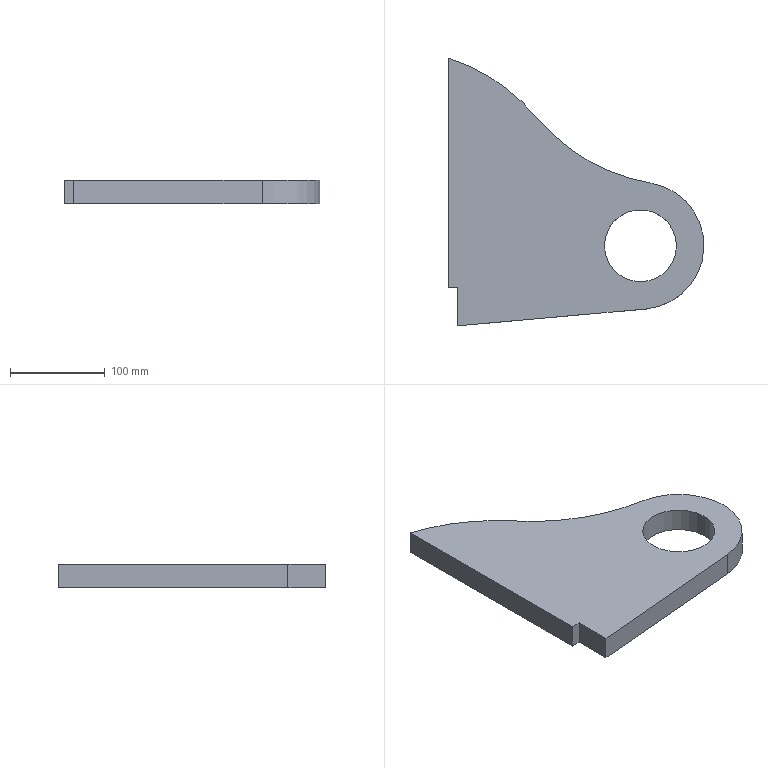Part | SolidWorks | features Extrusion 1 | 1 solid | 11 faces | box 270 x 282.5 x 25 mm | volume 1101150 mm3 | plane 6 | cylinder 5 | commonest cylinder face diameters 76 x2 400 x2 134 x1
STEP:
#1=CARTESIAN_POINT('',(-38.,0.,25.));
#2=VERTEX_POINT('',#1);
#3=CARTESIAN_POINT('',(38.,0.,25.));
#4=VERTEX_POINT('',#3);
#5=CARTESIAN_POINT('',(0.,0.,25.));
#6=DIRECTION('',(0.,0.,1.));
#7=DIRECTION('',(1.,0.,0.));
#8=AXIS2_PLACEMENT_3D('',#5,#6,#7);
#9=CIRCLE('',#8,38.);
#10=EDGE_CURVE('',#2,#4,#9,.T.);
#11=ORIENTED_EDGE('',*,*,#10,.T.);
#12=CARTESIAN_POINT('',(38.,0.,0.));
#13=VERTEX_POINT('',#12);
#14=CARTESIAN_POINT('',(38.,0.,25.));
#15=DIRECTION('',(0.,0.,-1.));
#16=VECTOR('',#15,1000.);
#17=LINE('',#14,#16);
#18=EDGE_CURVE('',#4,#13,#17,.T.);
#19=ORIENTED_EDGE('',*,*,#18,.T.);
#20=CARTESIAN_POINT('',(-38.,0.,0.));
#21=VERTEX_POINT('',#20);
#22=CARTESIAN_POINT('',(0.,0.,0.));
#23=DIRECTION('',(0.,0.,1.));
#24=DIRECTION('',(1.,0.,0.));
#25=AXIS2_PLACEMENT_3D('',#22,#23,#24);
#26=CIRCLE('',#25,38.);
#27=EDGE_CURVE('',#21,#13,#26,.T.);
#28=ORIENTED_EDGE('',*,*,#27,.F.);
#29=CARTESIAN_POINT('',(-38.,0.,25.));
#30=DIRECTION('',(0.,0.,-1.));
#31=VECTOR('',#30,1000.);
#32=LINE('',#29,#31);
#33=EDGE_CURVE('',#2,#21,#32,.T.);
#34=ORIENTED_EDGE('',*,*,#33,.F.);
#35=EDGE_LOOP('',(#11,#19,#28,#34));
#36=FACE_OUTER_BOUND('',#35,.T.);
#37=CARTESIAN_POINT('',(0.,0.,25.));
#38=DIRECTION('',(0.,0.,-1.));
#39=DIRECTION('',(-1.,0.,0.));
#40=AXIS2_PLACEMENT_3D('',#37,#38,#39);
#41=CYLINDRICAL_SURFACE('',#40,38.);
#42=ADVANCED_FACE('',(#36),#41,.F.);
#43=CARTESIAN_POINT('',(-109.363,135.258,25.));
#44=VERTEX_POINT('',#43);
#45=CARTESIAN_POINT('',(-203.,198.,25.));
#46=VERTEX_POINT('',#45);
#47=CARTESIAN_POINT('',(-263.,7.212,25.));
#48=DIRECTION('',(0.,0.,1.));
#49=DIRECTION('',(1.,0.,0.));
#50=AXIS2_PLACEMENT_3D('',#47,#48,#49);
#51=CIRCLE('',#50,200.);
#52=EDGE_CURVE('',#44,#46,#51,.T.);
#53=ORIENTED_EDGE('',*,*,#52,.T.);
#54=CARTESIAN_POINT('',(-203.,-44.5,25.));
#55=VERTEX_POINT('',#54);
#56=CARTESIAN_POINT('',(-203.,198.,25.));
#57=DIRECTION('',(0.,-1.,0.));
#58=VECTOR('',#57,1000.);
#59=LINE('',#56,#58);
#60=EDGE_CURVE('',#46,#55,#59,.T.);
#61=ORIENTED_EDGE('',*,*,#60,.T.);
#62=CARTESIAN_POINT('',(-193.,-44.5,25.));
#63=VERTEX_POINT('',#62);
#64=CARTESIAN_POINT('',(-203.,-44.5,25.));
#65=DIRECTION('',(1.,0.,0.));
#66=VECTOR('',#65,1000.);
#67=LINE('',#64,#66);
#68=EDGE_CURVE('',#55,#63,#67,.T.);
#69=ORIENTED_EDGE('',*,*,#68,.T.);
#70=CARTESIAN_POINT('',(-193.,-84.5,25.));
#71=VERTEX_POINT('',#70);
#72=CARTESIAN_POINT('',(-193.,-44.5,25.));
#73=DIRECTION('',(0.,-1.,0.));
#74=VECTOR('',#73,1000.);
#75=LINE('',#72,#74);
#76=EDGE_CURVE('',#63,#71,#75,.T.);
#77=ORIENTED_EDGE('',*,*,#76,.T.);
#78=CARTESIAN_POINT('',(5.959,-66.734,25.));
#79=VERTEX_POINT('',#78);
#80=CARTESIAN_POINT('',(-193.,-84.5,25.));
#81=DIRECTION('',(0.996,0.08894,0.));
#82=VECTOR('',#81,1000.);
#83=LINE('',#80,#82);
#84=EDGE_CURVE('',#71,#79,#83,.T.);
#85=ORIENTED_EDGE('',*,*,#84,.T.);
#86=CARTESIAN_POINT('',(11.11,66.072,25.));
#87=VERTEX_POINT('',#86);
#88=CARTESIAN_POINT('',(0.,0.,25.));
#89=DIRECTION('',(0.,0.,1.));
#90=DIRECTION('',(1.,0.,0.));
#91=AXIS2_PLACEMENT_3D('',#88,#89,#90);
#92=CIRCLE('',#91,67.);
#93=EDGE_CURVE('',#79,#87,#92,.T.);
#94=ORIENTED_EDGE('',*,*,#93,.T.);
#95=CARTESIAN_POINT('',(44.274,263.304,25.));
#96=DIRECTION('',(0.,0.,-1.));
#97=DIRECTION('',(1.,0.,0.));
#98=AXIS2_PLACEMENT_3D('',#95,#96,#97);
#99=CIRCLE('',#98,200.);
#100=EDGE_CURVE('',#87,#44,#99,.T.);
#101=ORIENTED_EDGE('',*,*,#100,.T.);
#102=EDGE_LOOP('',(#53,#61,#69,#77,#85,#94,#101));
#103=FACE_OUTER_BOUND('',#102,.T.);
#104=ORIENTED_EDGE('',*,*,#10,.F.);
#105=CARTESIAN_POINT('',(0.,0.,25.));
#106=DIRECTION('',(0.,0.,1.));
#107=DIRECTION('',(1.,0.,0.));
#108=AXIS2_PLACEMENT_3D('',#105,#106,#107);
#109=CIRCLE('',#108,38.);
#110=EDGE_CURVE('',#4,#2,#109,.T.);
#111=ORIENTED_EDGE('',*,*,#110,.F.);
#112=EDGE_LOOP('',(#104,#111));
#113=FACE_BOUND('',#112,.T.);
#114=CARTESIAN_POINT('',(-263.,7.212,25.));
#115=DIRECTION('',(0.,0.,1.));
#116=DIRECTION('',(1.,0.,0.));
#117=AXIS2_PLACEMENT_3D('',#114,#115,#116);
#118=PLANE('',#117);
#119=ADVANCED_FACE('',(#103,#113),#118,.T.);
#120=CARTESIAN_POINT('',(-109.363,135.258,0.));
#121=VERTEX_POINT('',#120);
#122=CARTESIAN_POINT('',(-203.,198.,0.));
#123=VERTEX_POINT('',#122);
#124=CARTESIAN_POINT('',(-263.,7.212,0.));
#125=DIRECTION('',(0.,0.,1.));
#126=DIRECTION('',(1.,0.,0.));
#127=AXIS2_PLACEMENT_3D('',#124,#125,#126);
#128=CIRCLE('',#127,200.);
#129=EDGE_CURVE('',#121,#123,#128,.T.);
#130=ORIENTED_EDGE('',*,*,#129,.F.);
#131=CARTESIAN_POINT('',(11.11,66.072,0.));
#132=VERTEX_POINT('',#131);
#133=CARTESIAN_POINT('',(44.274,263.304,0.));
#134=DIRECTION('',(0.,0.,-1.));
#135=DIRECTION('',(1.,0.,0.));
#136=AXIS2_PLACEMENT_3D('',#133,#134,#135);
#137=CIRCLE('',#136,200.);
#138=EDGE_CURVE('',#132,#121,#137,.T.);
#139=ORIENTED_EDGE('',*,*,#138,.F.);
#140=CARTESIAN_POINT('',(5.959,-66.734,0.));
#141=VERTEX_POINT('',#140);
#142=CARTESIAN_POINT('',(0.,0.,0.));
#143=DIRECTION('',(0.,0.,1.));
#144=DIRECTION('',(1.,0.,0.));
#145=AXIS2_PLACEMENT_3D('',#142,#143,#144);
#146=CIRCLE('',#145,67.);
#147=EDGE_CURVE('',#141,#132,#146,.T.);
#148=ORIENTED_EDGE('',*,*,#147,.F.);
#149=CARTESIAN_POINT('',(-193.,-84.5,0.));
#150=VERTEX_POINT('',#149);
#151=CARTESIAN_POINT('',(-193.,-84.5,0.));
#152=DIRECTION('',(0.996,0.08894,0.));
#153=VECTOR('',#152,1000.);
#154=LINE('',#151,#153);
#155=EDGE_CURVE('',#150,#141,#154,.T.);
#156=ORIENTED_EDGE('',*,*,#155,.F.);
#157=CARTESIAN_POINT('',(-193.,-44.5,0.));
#158=VERTEX_POINT('',#157);
#159=CARTESIAN_POINT('',(-193.,-44.5,0.));
#160=DIRECTION('',(0.,-1.,0.));
#161=VECTOR('',#160,1000.);
#162=LINE('',#159,#161);
#163=EDGE_CURVE('',#158,#150,#162,.T.);
#164=ORIENTED_EDGE('',*,*,#163,.F.);
#165=CARTESIAN_POINT('',(-203.,-44.5,0.));
#166=VERTEX_POINT('',#165);
#167=CARTESIAN_POINT('',(-203.,-44.5,0.));
#168=DIRECTION('',(1.,0.,0.));
#169=VECTOR('',#168,1000.);
#170=LINE('',#167,#169);
#171=EDGE_CURVE('',#166,#158,#170,.T.);
#172=ORIENTED_EDGE('',*,*,#171,.F.);
#173=CARTESIAN_POINT('',(-203.,198.,0.));
#174=DIRECTION('',(0.,-1.,0.));
#175=VECTOR('',#174,1000.);
#176=LINE('',#173,#175);
#177=EDGE_CURVE('',#123,#166,#176,.T.);
#178=ORIENTED_EDGE('',*,*,#177,.F.);
#179=EDGE_LOOP('',(#130,#139,#148,#156,#164,#172,#178));
#180=FACE_OUTER_BOUND('',#179,.T.);
#181=ORIENTED_EDGE('',*,*,#27,.T.);
#182=CARTESIAN_POINT('',(0.,0.,0.));
#183=DIRECTION('',(0.,0.,1.));
#184=DIRECTION('',(1.,0.,0.));
#185=AXIS2_PLACEMENT_3D('',#182,#183,#184);
#186=CIRCLE('',#185,38.);
#187=EDGE_CURVE('',#13,#21,#186,.T.);
#188=ORIENTED_EDGE('',*,*,#187,.T.);
#189=EDGE_LOOP('',(#181,#188));
#190=FACE_BOUND('',#189,.T.);
#191=CARTESIAN_POINT('',(-263.,7.212,0.));
#192=DIRECTION('',(0.,0.,1.));
#193=DIRECTION('',(1.,0.,0.));
#194=AXIS2_PLACEMENT_3D('',#191,#192,#193);
#195=PLANE('',#194);
#196=ADVANCED_FACE('',(#180,#190),#195,.F.);
#197=ORIENTED_EDGE('',*,*,#129,.T.);
#198=CARTESIAN_POINT('',(-203.,198.,25.));
#199=DIRECTION('',(0.,0.,-1.));
#200=VECTOR('',#199,1000.);
#201=LINE('',#198,#200);
#202=EDGE_CURVE('',#46,#123,#201,.T.);
#203=ORIENTED_EDGE('',*,*,#202,.F.);
#204=ORIENTED_EDGE('',*,*,#52,.F.);
#205=CARTESIAN_POINT('',(-109.363,135.258,25.));
#206=DIRECTION('',(0.,0.,-1.));
#207=VECTOR('',#206,1000.);
#208=LINE('',#205,#207);
#209=EDGE_CURVE('',#44,#121,#208,.T.);
#210=ORIENTED_EDGE('',*,*,#209,.T.);
#211=EDGE_LOOP('',(#197,#203,#204,#210));
#212=FACE_OUTER_BOUND('',#211,.T.);
#213=CARTESIAN_POINT('',(-263.,7.212,25.));
#214=DIRECTION('',(0.,0.,-1.));
#215=DIRECTION('',(-1.,0.,0.));
#216=AXIS2_PLACEMENT_3D('',#213,#214,#215);
#217=CYLINDRICAL_SURFACE('',#216,200.);
#218=ADVANCED_FACE('',(#212),#217,.T.);
#219=ORIENTED_EDGE('',*,*,#177,.T.);
#220=CARTESIAN_POINT('',(-203.,-44.5,25.));
#221=DIRECTION('',(0.,0.,-1.));
#222=VECTOR('',#221,1000.);
#223=LINE('',#220,#222);
#224=EDGE_CURVE('',#55,#166,#223,.T.);
#225=ORIENTED_EDGE('',*,*,#224,.F.);
#226=ORIENTED_EDGE('',*,*,#60,.F.);
#227=ORIENTED_EDGE('',*,*,#202,.T.);
#228=EDGE_LOOP('',(#219,#225,#226,#227));
#229=FACE_OUTER_BOUND('',#228,.T.);
#230=CARTESIAN_POINT('',(-203.,198.,25.));
#231=DIRECTION('',(1.,0.,0.));
#232=DIRECTION('',(0.,1.,0.));
#233=AXIS2_PLACEMENT_3D('',#230,#231,#232);
#234=PLANE('',#233);
#235=ADVANCED_FACE('',(#229),#234,.F.);
#236=ORIENTED_EDGE('',*,*,#171,.T.);
#237=CARTESIAN_POINT('',(-193.,-44.5,25.));
#238=DIRECTION('',(0.,0.,-1.));
#239=VECTOR('',#238,1000.);
#240=LINE('',#237,#239);
#241=EDGE_CURVE('',#63,#158,#240,.T.);
#242=ORIENTED_EDGE('',*,*,#241,.F.);
#243=ORIENTED_EDGE('',*,*,#68,.F.);
#244=ORIENTED_EDGE('',*,*,#224,.T.);
#245=EDGE_LOOP('',(#236,#242,#243,#244));
#246=FACE_OUTER_BOUND('',#245,.T.);
#247=CARTESIAN_POINT('',(-203.,-44.5,25.));
#248=DIRECTION('',(0.,1.,0.));
#249=DIRECTION('',(0.,0.,1.));
#250=AXIS2_PLACEMENT_3D('',#247,#248,#249);
#251=PLANE('',#250);
#252=ADVANCED_FACE('',(#246),#251,.F.);
#253=ORIENTED_EDGE('',*,*,#163,.T.);
#254=CARTESIAN_POINT('',(-193.,-84.5,25.));
#255=DIRECTION('',(0.,0.,-1.));
#256=VECTOR('',#255,1000.);
#257=LINE('',#254,#256);
#258=EDGE_CURVE('',#71,#150,#257,.T.);
#259=ORIENTED_EDGE('',*,*,#258,.F.);
#260=ORIENTED_EDGE('',*,*,#76,.F.);
#261=ORIENTED_EDGE('',*,*,#241,.T.);
#262=EDGE_LOOP('',(#253,#259,#260,#261));
#263=FACE_OUTER_BOUND('',#262,.T.);
#264=CARTESIAN_POINT('',(-193.,-44.5,25.));
#265=DIRECTION('',(1.,0.,0.));
#266=DIRECTION('',(0.,0.,-1.));
#267=AXIS2_PLACEMENT_3D('',#264,#265,#266);
#268=PLANE('',#267);
#269=ADVANCED_FACE('',(#263),#268,.F.);
#270=ORIENTED_EDGE('',*,*,#155,.T.);
#271=CARTESIAN_POINT('',(5.959,-66.734,25.));
#272=DIRECTION('',(0.,0.,-1.));
#273=VECTOR('',#272,1000.);
#274=LINE('',#271,#273);
#275=EDGE_CURVE('',#79,#141,#274,.T.);
#276=ORIENTED_EDGE('',*,*,#275,.F.);
#277=ORIENTED_EDGE('',*,*,#84,.F.);
#278=ORIENTED_EDGE('',*,*,#258,.T.);
#279=EDGE_LOOP('',(#270,#276,#277,#278));
#280=FACE_OUTER_BOUND('',#279,.T.);
#281=CARTESIAN_POINT('',(-193.,-84.5,25.));
#282=DIRECTION('',(-0.08894,0.996,0.));
#283=DIRECTION('',(-0.996,-0.08894,0.));
#284=AXIS2_PLACEMENT_3D('',#281,#282,#283);
#285=PLANE('',#284);
#286=ADVANCED_FACE('',(#280),#285,.F.);
#287=ORIENTED_EDGE('',*,*,#147,.T.);
#288=CARTESIAN_POINT('',(11.11,66.072,25.));
#289=DIRECTION('',(0.,0.,-1.));
#290=VECTOR('',#289,1000.);
#291=LINE('',#288,#290);
#292=EDGE_CURVE('',#87,#132,#291,.T.);
#293=ORIENTED_EDGE('',*,*,#292,.F.);
#294=ORIENTED_EDGE('',*,*,#93,.F.);
#295=ORIENTED_EDGE('',*,*,#275,.T.);
#296=EDGE_LOOP('',(#287,#293,#294,#295));
#297=FACE_OUTER_BOUND('',#296,.T.);
#298=CARTESIAN_POINT('',(0.,0.,25.));
#299=DIRECTION('',(0.,0.,-1.));
#300=DIRECTION('',(-1.,0.,0.));
#301=AXIS2_PLACEMENT_3D('',#298,#299,#300);
#302=CYLINDRICAL_SURFACE('',#301,67.);
#303=ADVANCED_FACE('',(#297),#302,.T.);
#304=ORIENTED_EDGE('',*,*,#138,.T.);
#305=ORIENTED_EDGE('',*,*,#209,.F.);
#306=ORIENTED_EDGE('',*,*,#100,.F.);
#307=ORIENTED_EDGE('',*,*,#292,.T.);
#308=EDGE_LOOP('',(#304,#305,#306,#307));
#309=FACE_OUTER_BOUND('',#308,.T.);
#310=CARTESIAN_POINT('',(44.274,263.304,25.));
#311=DIRECTION('',(0.,0.,-1.));
#312=DIRECTION('',(-1.,0.,0.));
#313=AXIS2_PLACEMENT_3D('',#310,#311,#312);
#314=CYLINDRICAL_SURFACE('',#313,200.);
#315=ADVANCED_FACE('',(#309),#314,.F.);
#316=ORIENTED_EDGE('',*,*,#18,.F.);
#317=ORIENTED_EDGE('',*,*,#110,.T.);
#318=ORIENTED_EDGE('',*,*,#33,.T.);
#319=ORIENTED_EDGE('',*,*,#187,.F.);
#320=EDGE_LOOP('',(#316,#317,#318,#319));
#321=FACE_OUTER_BOUND('',#320,.T.);
#322=CARTESIAN_POINT('',(0.,0.,25.));
#323=DIRECTION('',(0.,0.,-1.));
#324=DIRECTION('',(-1.,0.,0.));
#325=AXIS2_PLACEMENT_3D('',#322,#323,#324);
#326=CYLINDRICAL_SURFACE('',#325,38.);
#327=ADVANCED_FACE('',(#321),#326,.F.);
#328=CLOSED_SHELL('',(#42,#119,#196,#218,#235,#252,#269,#286,#303,#315,#327));
#329=MANIFOLD_SOLID_BREP('',#328);
#330=CARTESIAN_POINT('',(0.,0.,0.));
#331=DIRECTION('',(0.,0.,1.));
#332=DIRECTION('',(1.,0.,0.));
#333=AXIS2_PLACEMENT_3D('',#330,#331,#332);
#334=(LENGTH_UNIT()NAMED_UNIT(*)SI_UNIT(.MILLI.,.METRE.));
#335=UNCERTAINTY_MEASURE_WITH_UNIT(LENGTH_MEASURE(0.00001),#334,'','');
#336=(NAMED_UNIT(*)PLANE_ANGLE_UNIT()SI_UNIT($,.RADIAN.));
#337=(NAMED_UNIT(*)SI_UNIT($,.STERADIAN.)SOLID_ANGLE_UNIT());
#338=(GEOMETRIC_REPRESENTATION_CONTEXT(3)GLOBAL_UNCERTAINTY_ASSIGNED_CONTEXT((#335))GLOBAL_UNIT_ASSIGNED_CONTEXT((#334,#336,#337))REPRESENTATION_CONTEXT('',''));
#339=ADVANCED_BREP_SHAPE_REPRESENTATION('',(#329,#333),#338);